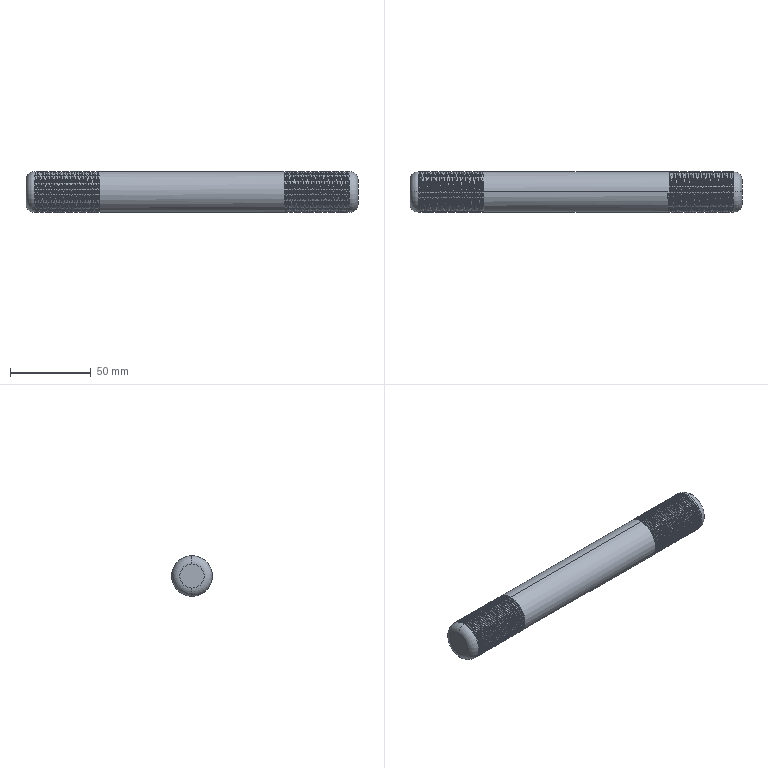Part | SolidWorks | features SweepThread 2, Fillet 1, Revolution 1 | 1 solid | 178 faces | box 205 x 25 x 25 mm | volume 98310 mm3 | cylinder 162 | plane 6 | spline 6 | torus 4 | commonest cylinder face diameters 25 x162